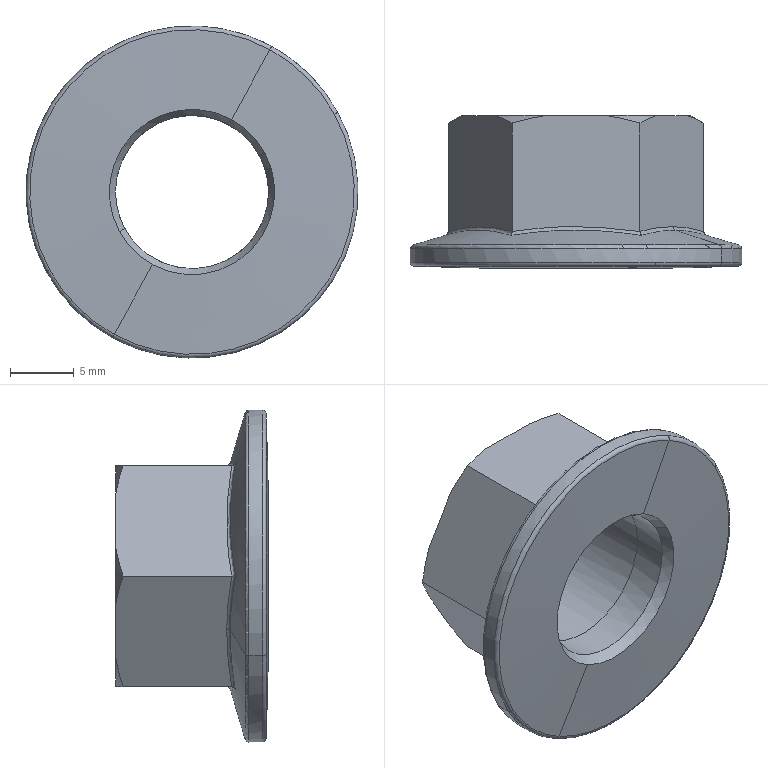Part | NX | features BREP 1 | 1 solid | 42 faces | box 26 x 11.959 x 26 mm | volume 2329 mm3 | cone 14 | spline 8 | plane 7 | torus 7 | cylinder 6 | commonest cylinder face diameters 12 x4 26 x2